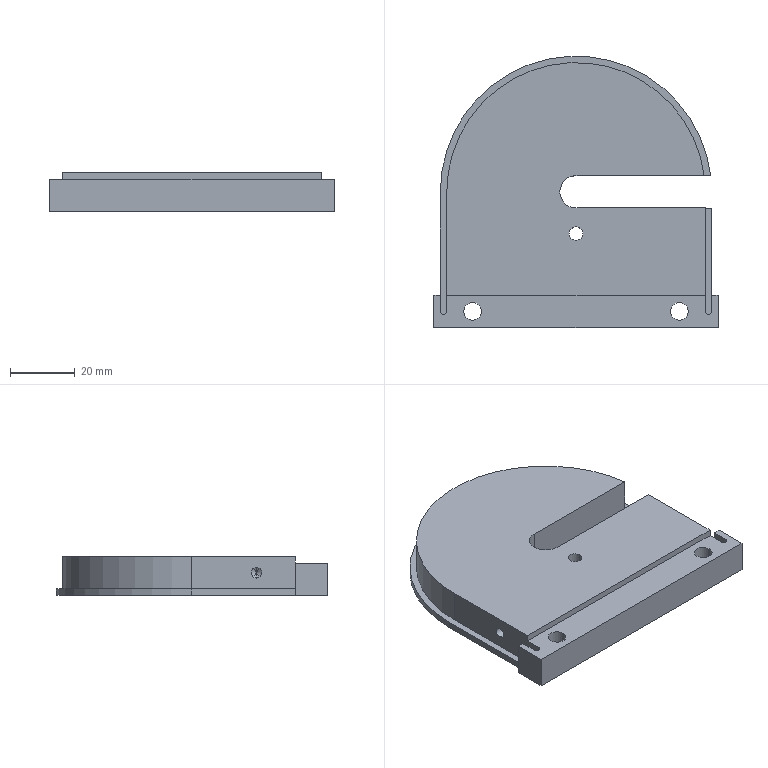Part | SolidWorks | features ICE 6, 3DProfileFeature 3, HoleWzd 3, Extrusion 1 | 1 solid | 45 faces | box 88 x 84 x 12 mm | volume 63664 mm3 | plane 21 | cylinder 20 | cone 4 | commonest cylinder face diameters 3.3 x4 5.5 x4 9 x4 2 x2 4.2 x2 10 x2
STEP:
#1=CARTESIAN_POINT('',(2.1,8.082,12.));
#2=VERTEX_POINT('',#1);
#3=CARTESIAN_POINT('',(-2.1,8.082,12.));
#4=VERTEX_POINT('',#3);
#5=CARTESIAN_POINT('',(0.,8.082,12.));
#6=DIRECTION('',(0.,0.,-1.));
#7=DIRECTION('',(-1.,0.,0.));
#8=AXIS2_PLACEMENT_3D('',#5,#6,#7);
#9=CIRCLE('',#8,2.1);
#10=EDGE_CURVE('',#2,#4,#9,.T.);
#11=ORIENTED_EDGE('',*,*,#10,.F.);
#12=CARTESIAN_POINT('',(2.1,8.082,0.));
#13=VERTEX_POINT('',#12);
#14=CARTESIAN_POINT('',(2.1,8.082,0.));
#15=DIRECTION('',(0.,0.,-1.));
#16=VECTOR('',#15,1000.);
#17=LINE('',#14,#16);
#18=EDGE_CURVE('',#2,#13,#17,.T.);
#19=ORIENTED_EDGE('',*,*,#18,.T.);
#20=CARTESIAN_POINT('',(-2.1,8.082,0.));
#21=VERTEX_POINT('',#20);
#22=CARTESIAN_POINT('',(0.,8.082,0.));
#23=DIRECTION('',(0.,0.,-1.));
#24=DIRECTION('',(-1.,0.,0.));
#25=AXIS2_PLACEMENT_3D('',#22,#23,#24);
#26=CIRCLE('',#25,2.1);
#27=EDGE_CURVE('',#13,#21,#26,.T.);
#28=ORIENTED_EDGE('',*,*,#27,.T.);
#29=CARTESIAN_POINT('',(-2.1,8.082,0.));
#30=DIRECTION('',(0.,0.,-1.));
#31=VECTOR('',#30,1000.);
#32=LINE('',#29,#31);
#33=EDGE_CURVE('',#4,#21,#32,.T.);
#34=ORIENTED_EDGE('',*,*,#33,.F.);
#35=EDGE_LOOP('',(#11,#19,#28,#34));
#36=FACE_OUTER_BOUND('',#35,.T.);
#37=CARTESIAN_POINT('',(0.,8.082,0.));
#38=DIRECTION('',(0.,0.,-1.));
#39=DIRECTION('',(-1.,0.,0.));
#40=AXIS2_PLACEMENT_3D('',#37,#38,#39);
#41=CYLINDRICAL_SURFACE('',#40,2.1);
#42=ADVANCED_FACE('',(#36),#41,.F.);
#43=CARTESIAN_POINT('',(30.,1.,8.665));
#44=VERTEX_POINT('',#43);
#45=CARTESIAN_POINT('',(30.,1.,5.365));
#46=VERTEX_POINT('',#45);
#47=CARTESIAN_POINT('',(30.,1.,7.015));
#48=DIRECTION('',(1.,0.,0.));
#49=DIRECTION('',(0.,0.,-1.));
#50=AXIS2_PLACEMENT_3D('',#47,#48,#49);
#51=CIRCLE('',#50,1.65);
#52=EDGE_CURVE('',#44,#46,#51,.T.);
#53=ORIENTED_EDGE('',*,*,#52,.F.);
#54=CARTESIAN_POINT('',(40.,1.,8.665));
#55=VERTEX_POINT('',#54);
#56=CARTESIAN_POINT('',(40.,1.,8.665));
#57=DIRECTION('',(1.,0.,0.));
#58=VECTOR('',#57,1000.);
#59=LINE('',#56,#58);
#60=EDGE_CURVE('',#44,#55,#59,.T.);
#61=ORIENTED_EDGE('',*,*,#60,.T.);
#62=CARTESIAN_POINT('',(40.,1.,5.365));
#63=VERTEX_POINT('',#62);
#64=CARTESIAN_POINT('',(40.,1.,7.015));
#65=DIRECTION('',(1.,0.,0.));
#66=DIRECTION('',(0.,0.,-1.));
#67=AXIS2_PLACEMENT_3D('',#64,#65,#66);
#68=CIRCLE('',#67,1.65);
#69=EDGE_CURVE('',#55,#63,#68,.T.);
#70=ORIENTED_EDGE('',*,*,#69,.T.);
#71=CARTESIAN_POINT('',(40.,1.,5.365));
#72=DIRECTION('',(1.,0.,0.));
#73=VECTOR('',#72,1000.);
#74=LINE('',#71,#73);
#75=EDGE_CURVE('',#46,#63,#74,.T.);
#76=ORIENTED_EDGE('',*,*,#75,.F.);
#77=EDGE_LOOP('',(#53,#61,#70,#76));
#78=FACE_OUTER_BOUND('',#77,.T.);
#79=CARTESIAN_POINT('',(40.,1.,7.015));
#80=DIRECTION('',(1.,0.,0.));
#81=DIRECTION('',(0.,0.,-1.));
#82=AXIS2_PLACEMENT_3D('',#79,#80,#81);
#83=CYLINDRICAL_SURFACE('',#82,1.65);
#84=ADVANCED_FACE('',(#78),#83,.F.);
#85=CARTESIAN_POINT('',(29.009,1.,7.015));
#86=VERTEX_POINT('',#85);
#87=CARTESIAN_POINT('',(30.,1.,5.365));
#88=DIRECTION('',(0.515,0.,-0.8572));
#89=VECTOR('',#88,1000.);
#90=LINE('',#87,#89);
#91=EDGE_CURVE('',#86,#46,#90,.T.);
#92=ORIENTED_EDGE('',*,*,#91,.F.);
#93=CARTESIAN_POINT('',(30.,1.,8.665));
#94=DIRECTION('',(0.515,0.,0.8572));
#95=VECTOR('',#94,1000.);
#96=LINE('',#93,#95);
#97=EDGE_CURVE('',#86,#44,#96,.T.);
#98=ORIENTED_EDGE('',*,*,#97,.T.);
#99=ORIENTED_EDGE('',*,*,#52,.T.);
#100=EDGE_LOOP('',(#92,#98,#99));
#101=FACE_OUTER_BOUND('',#100,.T.);
#102=CARTESIAN_POINT('',(30.,1.,7.015));
#103=DIRECTION('',(1.,0.,0.));
#104=DIRECTION('',(0.,0.,-1.));
#105=AXIS2_PLACEMENT_3D('',#102,#103,#104);
#106=CONICAL_SURFACE('',#105,1.65,1.03);
#107=ADVANCED_FACE('',(#101),#106,.F.);
#108=CARTESIAN_POINT('',(-30.,1.,5.35));
#109=VERTEX_POINT('',#108);
#110=CARTESIAN_POINT('',(-30.,1.,8.65));
#111=VERTEX_POINT('',#110);
#112=CARTESIAN_POINT('',(-30.,1.,7.));
#113=DIRECTION('',(-1.,0.,0.));
#114=DIRECTION('',(0.,0.,1.));
#115=AXIS2_PLACEMENT_3D('',#112,#113,#114);
#116=CIRCLE('',#115,1.65);
#117=EDGE_CURVE('',#109,#111,#116,.T.);
#118=ORIENTED_EDGE('',*,*,#117,.F.);
#119=CARTESIAN_POINT('',(-40.,1.,5.35));
#120=VERTEX_POINT('',#119);
#121=CARTESIAN_POINT('',(-40.,1.,5.35));
#122=DIRECTION('',(-1.,0.,0.));
#123=VECTOR('',#122,1000.);
#124=LINE('',#121,#123);
#125=EDGE_CURVE('',#109,#120,#124,.T.);
#126=ORIENTED_EDGE('',*,*,#125,.T.);
#127=CARTESIAN_POINT('',(-40.,1.,8.65));
#128=VERTEX_POINT('',#127);
#129=CARTESIAN_POINT('',(-40.,1.,7.));
#130=DIRECTION('',(-1.,0.,0.));
#131=DIRECTION('',(0.,0.,1.));
#132=AXIS2_PLACEMENT_3D('',#129,#130,#131);
#133=CIRCLE('',#132,1.65);
#134=EDGE_CURVE('',#120,#128,#133,.T.);
#135=ORIENTED_EDGE('',*,*,#134,.T.);
#136=CARTESIAN_POINT('',(-40.,1.,8.65));
#137=DIRECTION('',(-1.,0.,0.));
#138=VECTOR('',#137,1000.);
#139=LINE('',#136,#138);
#140=EDGE_CURVE('',#111,#128,#139,.T.);
#141=ORIENTED_EDGE('',*,*,#140,.F.);
#142=EDGE_LOOP('',(#118,#126,#135,#141));
#143=FACE_OUTER_BOUND('',#142,.T.);
#144=CARTESIAN_POINT('',(-40.,1.,7.));
#145=DIRECTION('',(-1.,0.,0.));
#146=DIRECTION('',(0.,0.,1.));
#147=AXIS2_PLACEMENT_3D('',#144,#145,#146);
#148=CYLINDRICAL_SURFACE('',#147,1.65);
#149=ADVANCED_FACE('',(#143),#148,.F.);
#150=CARTESIAN_POINT('',(-29.009,1.,7.));
#151=VERTEX_POINT('',#150);
#152=CARTESIAN_POINT('',(-30.,1.,8.65));
#153=DIRECTION('',(-0.515,0.,0.8572));
#154=VECTOR('',#153,1000.);
#155=LINE('',#152,#154);
#156=EDGE_CURVE('',#151,#111,#155,.T.);
#157=ORIENTED_EDGE('',*,*,#156,.F.);
#158=CARTESIAN_POINT('',(-30.,1.,5.35));
#159=DIRECTION('',(-0.515,0.,-0.8572));
#160=VECTOR('',#159,1000.);
#161=LINE('',#158,#160);
#162=EDGE_CURVE('',#151,#109,#161,.T.);
#163=ORIENTED_EDGE('',*,*,#162,.T.);
#164=ORIENTED_EDGE('',*,*,#117,.T.);
#165=EDGE_LOOP('',(#157,#163,#164));
#166=FACE_OUTER_BOUND('',#165,.T.);
#167=CARTESIAN_POINT('',(-30.,1.,7.));
#168=DIRECTION('',(-1.,0.,0.));
#169=DIRECTION('',(0.,0.,1.));
#170=AXIS2_PLACEMENT_3D('',#167,#168,#169);
#171=CONICAL_SURFACE('',#170,1.65,1.03);
#172=ADVANCED_FACE('',(#166),#171,.F.);
#173=CARTESIAN_POINT('',(-27.5,-16.,6.));
#174=VERTEX_POINT('',#173);
#175=CARTESIAN_POINT('',(-36.5,-16.,6.));
#176=VERTEX_POINT('',#175);
#177=CARTESIAN_POINT('',(-32.,-16.,6.));
#178=DIRECTION('',(0.,0.,-1.));
#179=DIRECTION('',(-1.,0.,0.));
#180=AXIS2_PLACEMENT_3D('',#177,#178,#179);
#181=CIRCLE('',#180,4.5);
#182=EDGE_CURVE('',#174,#176,#181,.T.);
#183=ORIENTED_EDGE('',*,*,#182,.F.);
#184=CARTESIAN_POINT('',(-27.5,-16.,0.));
#185=VERTEX_POINT('',#184);
#186=CARTESIAN_POINT('',(-27.5,-16.,6.));
#187=DIRECTION('',(0.,0.,-1.));
#188=VECTOR('',#187,1000.);
#189=LINE('',#186,#188);
#190=EDGE_CURVE('',#174,#185,#189,.T.);
#191=ORIENTED_EDGE('',*,*,#190,.T.);
#192=CARTESIAN_POINT('',(-36.5,-16.,0.));
#193=VERTEX_POINT('',#192);
#194=CARTESIAN_POINT('',(-32.,-16.,0.));
#195=DIRECTION('',(0.,0.,-1.));
#196=DIRECTION('',(-1.,0.,0.));
#197=AXIS2_PLACEMENT_3D('',#194,#195,#196);
#198=CIRCLE('',#197,4.5);
#199=EDGE_CURVE('',#185,#193,#198,.T.);
#200=ORIENTED_EDGE('',*,*,#199,.T.);
#201=CARTESIAN_POINT('',(-36.5,-16.,6.));
#202=DIRECTION('',(0.,0.,-1.));
#203=VECTOR('',#202,1000.);
#204=LINE('',#201,#203);
#205=EDGE_CURVE('',#176,#193,#204,.T.);
#206=ORIENTED_EDGE('',*,*,#205,.F.);
#207=EDGE_LOOP('',(#183,#191,#200,#206));
#208=FACE_OUTER_BOUND('',#207,.T.);
#209=CARTESIAN_POINT('',(-32.,-16.,6.));
#210=DIRECTION('',(0.,0.,-1.));
#211=DIRECTION('',(-1.,0.,0.));
#212=AXIS2_PLACEMENT_3D('',#209,#210,#211);
#213=CYLINDRICAL_SURFACE('',#212,4.5);
#214=ADVANCED_FACE('',(#208),#213,.F.);
#215=CARTESIAN_POINT('',(36.5,-16.,6.));
#216=VERTEX_POINT('',#215);
#217=CARTESIAN_POINT('',(27.5,-16.,6.));
#218=VERTEX_POINT('',#217);
#219=CARTESIAN_POINT('',(32.,-16.,6.));
#220=DIRECTION('',(0.,0.,-1.));
#221=DIRECTION('',(-1.,0.,0.));
#222=AXIS2_PLACEMENT_3D('',#219,#220,#221);
#223=CIRCLE('',#222,4.5);
#224=EDGE_CURVE('',#216,#218,#223,.T.);
#225=ORIENTED_EDGE('',*,*,#224,.F.);
#226=CARTESIAN_POINT('',(36.5,-16.,0.));
#227=VERTEX_POINT('',#226);
#228=CARTESIAN_POINT('',(36.5,-16.,6.));
#229=DIRECTION('',(0.,0.,-1.));
#230=VECTOR('',#229,1000.);
#231=LINE('',#228,#230);
#232=EDGE_CURVE('',#216,#227,#231,.T.);
#233=ORIENTED_EDGE('',*,*,#232,.T.);
#234=CARTESIAN_POINT('',(27.5,-16.,0.));
#235=VERTEX_POINT('',#234);
#236=CARTESIAN_POINT('',(32.,-16.,0.));
#237=DIRECTION('',(0.,0.,-1.));
#238=DIRECTION('',(-1.,0.,0.));
#239=AXIS2_PLACEMENT_3D('',#236,#237,#238);
#240=CIRCLE('',#239,4.5);
#241=EDGE_CURVE('',#227,#235,#240,.T.);
#242=ORIENTED_EDGE('',*,*,#241,.T.);
#243=CARTESIAN_POINT('',(27.5,-16.,6.));
#244=DIRECTION('',(0.,0.,-1.));
#245=VECTOR('',#244,1000.);
#246=LINE('',#243,#245);
#247=EDGE_CURVE('',#218,#235,#246,.T.);
#248=ORIENTED_EDGE('',*,*,#247,.F.);
#249=EDGE_LOOP('',(#225,#233,#242,#248));
#250=FACE_OUTER_BOUND('',#249,.T.);
#251=CARTESIAN_POINT('',(32.,-16.,6.));
#252=DIRECTION('',(0.,0.,-1.));
#253=DIRECTION('',(-1.,0.,0.));
#254=AXIS2_PLACEMENT_3D('',#251,#252,#253);
#255=CYLINDRICAL_SURFACE('',#254,4.5);
#256=ADVANCED_FACE('',(#250),#255,.F.);
#257=CARTESIAN_POINT('',(-5.,21.,12.));
#258=VERTEX_POINT('',#257);
#259=CARTESIAN_POINT('',(0.,26.,12.));
#260=VERTEX_POINT('',#259);
#261=CARTESIAN_POINT('',(0.,21.,12.));
#262=DIRECTION('',(0.,0.,-1.));
#263=DIRECTION('',(-1.,0.,0.));
#264=AXIS2_PLACEMENT_3D('',#261,#262,#263);
#265=CIRCLE('',#264,5.);
#266=EDGE_CURVE('',#258,#260,#265,.T.);
#267=ORIENTED_EDGE('',*,*,#266,.F.);
#268=CARTESIAN_POINT('',(-5.,21.,0.));
#269=VERTEX_POINT('',#268);
#270=CARTESIAN_POINT('',(-5.,21.,12.));
#271=DIRECTION('',(0.,0.,-1.));
#272=VECTOR('',#271,1000.);
#273=LINE('',#270,#272);
#274=EDGE_CURVE('',#258,#269,#273,.T.);
#275=ORIENTED_EDGE('',*,*,#274,.T.);
#276=CARTESIAN_POINT('',(0.,26.,0.));
#277=VERTEX_POINT('',#276);
#278=CARTESIAN_POINT('',(0.,21.,0.));
#279=DIRECTION('',(0.,0.,-1.));
#280=DIRECTION('',(-1.,0.,0.));
#281=AXIS2_PLACEMENT_3D('',#278,#279,#280);
#282=CIRCLE('',#281,5.);
#283=EDGE_CURVE('',#269,#277,#282,.T.);
#284=ORIENTED_EDGE('',*,*,#283,.T.);
#285=CARTESIAN_POINT('',(0.,26.,12.));
#286=DIRECTION('',(0.,0.,-1.));
#287=VECTOR('',#286,1000.);
#288=LINE('',#285,#287);
#289=EDGE_CURVE('',#260,#277,#288,.T.);
#290=ORIENTED_EDGE('',*,*,#289,.F.);
#291=EDGE_LOOP('',(#267,#275,#284,#290));
#292=FACE_OUTER_BOUND('',#291,.T.);
#293=CARTESIAN_POINT('',(0.,21.,12.));
#294=DIRECTION('',(0.,0.,-1.));
#295=DIRECTION('',(-1.,0.,0.));
#296=AXIS2_PLACEMENT_3D('',#293,#294,#295);
#297=CYLINDRICAL_SURFACE('',#296,5.);
#298=ADVANCED_FACE('',(#292),#297,.F.);
#299=CARTESIAN_POINT('',(34.75,-16.,10.));
#300=VERTEX_POINT('',#299);
#301=CARTESIAN_POINT('',(29.25,-16.,10.));
#302=VERTEX_POINT('',#301);
#303=CARTESIAN_POINT('',(32.,-16.,10.));
#304=DIRECTION('',(0.,0.,-1.));
#305=DIRECTION('',(-1.,0.,0.));
#306=AXIS2_PLACEMENT_3D('',#303,#304,#305);
#307=CIRCLE('',#306,2.75);
#308=EDGE_CURVE('',#300,#302,#307,.T.);
#309=ORIENTED_EDGE('',*,*,#308,.F.);
#310=CARTESIAN_POINT('',(34.75,-16.,6.));
#311=VERTEX_POINT('',#310);
#312=CARTESIAN_POINT('',(34.75,-16.,12.));
#313=DIRECTION('',(0.,0.,-1.));
#314=VECTOR('',#313,1000.);
#315=LINE('',#312,#314);
#316=EDGE_CURVE('',#300,#311,#315,.T.);
#317=ORIENTED_EDGE('',*,*,#316,.T.);
#318=CARTESIAN_POINT('',(29.25,-16.,6.));
#319=VERTEX_POINT('',#318);
#320=CARTESIAN_POINT('',(32.,-16.,6.));
#321=DIRECTION('',(0.,0.,1.));
#322=DIRECTION('',(-1.,0.,0.));
#323=AXIS2_PLACEMENT_3D('',#320,#321,#322);
#324=CIRCLE('',#323,2.75);
#325=EDGE_CURVE('',#319,#311,#324,.T.);
#326=ORIENTED_EDGE('',*,*,#325,.F.);
#327=CARTESIAN_POINT('',(29.25,-16.,12.));
#328=DIRECTION('',(0.,0.,-1.));
#329=VECTOR('',#328,1000.);
#330=LINE('',#327,#329);
#331=EDGE_CURVE('',#302,#319,#330,.T.);
#332=ORIENTED_EDGE('',*,*,#331,.F.);
#333=EDGE_LOOP('',(#309,#317,#326,#332));
#334=FACE_OUTER_BOUND('',#333,.T.);
#335=CARTESIAN_POINT('',(32.,-16.,12.));
#336=DIRECTION('',(0.,0.,-1.));
#337=DIRECTION('',(-1.,0.,0.));
#338=AXIS2_PLACEMENT_3D('',#335,#336,#337);
#339=CYLINDRICAL_SURFACE('',#338,2.75);
#340=ADVANCED_FACE('',(#334),#339,.F.);
#341=CARTESIAN_POINT('',(-29.25,-16.,10.));
#342=VERTEX_POINT('',#341);
#343=CARTESIAN_POINT('',(-34.75,-16.,10.));
#344=VERTEX_POINT('',#343);
#345=CARTESIAN_POINT('',(-32.,-16.,10.));
#346=DIRECTION('',(0.,0.,-1.));
#347=DIRECTION('',(-1.,0.,0.));
#348=AXIS2_PLACEMENT_3D('',#345,#346,#347);
#349=CIRCLE('',#348,2.75);
#350=EDGE_CURVE('',#342,#344,#349,.T.);
#351=ORIENTED_EDGE('',*,*,#350,.F.);
#352=CARTESIAN_POINT('',(-29.25,-16.,6.));
#353=VERTEX_POINT('',#352);
#354=CARTESIAN_POINT('',(-29.25,-16.,12.));
#355=DIRECTION('',(0.,0.,-1.));
#356=VECTOR('',#355,1000.);
#357=LINE('',#354,#356);
#358=EDGE_CURVE('',#342,#353,#357,.T.);
#359=ORIENTED_EDGE('',*,*,#358,.T.);
#360=CARTESIAN_POINT('',(-34.75,-16.,6.));
#361=VERTEX_POINT('',#360);
#362=CARTESIAN_POINT('',(-32.,-16.,6.));
#363=DIRECTION('',(0.,0.,1.));
#364=DIRECTION('',(-1.,0.,0.));
#365=AXIS2_PLACEMENT_3D('',#362,#363,#364);
#366=CIRCLE('',#365,2.75);
#367=EDGE_CURVE('',#361,#353,#366,.T.);
#368=ORIENTED_EDGE('',*,*,#367,.F.);
#369=CARTESIAN_POINT('',(-34.75,-16.,12.));
#370=DIRECTION('',(0.,0.,-1.));
#371=VECTOR('',#370,1000.);
#372=LINE('',#369,#371);
#373=EDGE_CURVE('',#344,#361,#372,.T.);
#374=ORIENTED_EDGE('',*,*,#373,.F.);
#375=EDGE_LOOP('',(#351,#359,#368,#374));
#376=FACE_OUTER_BOUND('',#375,.T.);
#377=CARTESIAN_POINT('',(-32.,-16.,12.));
#378=DIRECTION('',(0.,0.,-1.));
#379=DIRECTION('',(-1.,0.,0.));
#380=AXIS2_PLACEMENT_3D('',#377,#378,#379);
#381=CYLINDRICAL_SURFACE('',#380,2.75);
#382=ADVANCED_FACE('',(#376),#381,.F.);
#383=ORIENTED_EDGE('',*,*,#358,.F.);
#384=CARTESIAN_POINT('',(-32.,-16.,10.));
#385=DIRECTION('',(0.,0.,-1.));
#386=DIRECTION('',(-1.,0.,0.));
#387=AXIS2_PLACEMENT_3D('',#384,#385,#386);
#388=CIRCLE('',#387,2.75);
#389=EDGE_CURVE('',#344,#342,#388,.T.);
#390=ORIENTED_EDGE('',*,*,#389,.F.);
#391=ORIENTED_EDGE('',*,*,#373,.T.);
#392=CARTESIAN_POINT('',(-32.,-16.,6.));
#393=DIRECTION('',(0.,0.,1.));
#394=DIRECTION('',(-1.,0.,0.));
#395=AXIS2_PLACEMENT_3D('',#392,#393,#394);
#396=CIRCLE('',#395,2.75);
#397=EDGE_CURVE('',#353,#361,#396,.T.);
#398=ORIENTED_EDGE('',*,*,#397,.F.);
#399=EDGE_LOOP('',(#383,#390,#391,#398));
#400=FACE_OUTER_BOUND('',#399,.T.);
#401=CARTESIAN_POINT('',(-32.,-16.,12.));
#402=DIRECTION('',(0.,0.,-1.));
#403=DIRECTION('',(-1.,0.,0.));
#404=AXIS2_PLACEMENT_3D('',#401,#402,#403);
#405=CYLINDRICAL_SURFACE('',#404,2.75);
#406=ADVANCED_FACE('',(#400),#405,.F.);
#407=ORIENTED_EDGE('',*,*,#316,.F.);
#408=CARTESIAN_POINT('',(32.,-16.,10.));
#409=DIRECTION('',(0.,0.,-1.));
#410=DIRECTION('',(-1.,0.,0.));
#411=AXIS2_PLACEMENT_3D('',#408,#409,#410);
#412=CIRCLE('',#411,2.75);
#413=EDGE_CURVE('',#302,#300,#412,.T.);
#414=ORIENTED_EDGE('',*,*,#413,.F.);
#415=ORIENTED_EDGE('',*,*,#331,.T.);
#416=CARTESIAN_POINT('',(32.,-16.,6.));
#417=DIRECTION('',(0.,0.,1.));
#418=DIRECTION('',(-1.,0.,0.));
#419=AXIS2_PLACEMENT_3D('',#416,#417,#418);
#420=CIRCLE('',#419,2.75);
#421=EDGE_CURVE('',#311,#319,#420,.T.);
#422=ORIENTED_EDGE('',*,*,#421,.F.);
#423=EDGE_LOOP('',(#407,#414,#415,#422));
#424=FACE_OUTER_BOUND('',#423,.T.);
#425=CARTESIAN_POINT('',(32.,-16.,12.));
#426=DIRECTION('',(0.,0.,-1.));
#427=DIRECTION('',(-1.,0.,0.));
#428=AXIS2_PLACEMENT_3D('',#425,#426,#427);
#429=CYLINDRICAL_SURFACE('',#428,2.75);
#430=ADVANCED_FACE('',(#424),#429,.F.);
#431=CARTESIAN_POINT('',(40.,16.,2.));
#432=VERTEX_POINT('',#431);
#433=CARTESIAN_POINT('',(42.,16.,2.));
#434=VERTEX_POINT('',#433);
#435=CARTESIAN_POINT('',(0.,16.,2.));
#436=DIRECTION('',(1.,0.,0.));
#437=VECTOR('',#436,1000.);
#438=LINE('',#435,#437);
#439=EDGE_CURVE('',#432,#434,#438,.T.);
#440=ORIENTED_EDGE('',*,*,#439,.F.);
#441=CARTESIAN_POINT('',(40.,-16.,2.));
#442=VERTEX_POINT('',#441);
#443=CARTESIAN_POINT('',(40.,-11.,2.));
#444=DIRECTION('',(0.,-1.,0.));
#445=VECTOR('',#444,1000.);
#446=LINE('',#443,#445);
#447=EDGE_CURVE('',#432,#442,#446,.T.);
#448=ORIENTED_EDGE('',*,*,#447,.T.);
#449=CARTESIAN_POINT('',(42.,-16.,2.));
#450=VERTEX_POINT('',#449);
#451=CARTESIAN_POINT('',(41.,-16.,2.));
#452=DIRECTION('',(0.,0.,1.));
#453=DIRECTION('',(1.,0.,0.));
#454=AXIS2_PLACEMENT_3D('',#451,#452,#453);
#455=CIRCLE('',#454,1.);
#456=EDGE_CURVE('',#442,#450,#455,.T.);
#457=ORIENTED_EDGE('',*,*,#456,.T.);
#458=CARTESIAN_POINT('',(42.,-11.,2.));
#459=VERTEX_POINT('',#458);
#460=CARTESIAN_POINT('',(42.,-11.,2.));
#461=DIRECTION('',(0.,1.,0.));
#462=VECTOR('',#461,1000.);
#463=LINE('',#460,#462);
#464=EDGE_CURVE('',#450,#459,#463,.T.);
#465=ORIENTED_EDGE('',*,*,#464,.T.);
#466=CARTESIAN_POINT('',(42.,21.,2.));
#467=DIRECTION('',(0.,1.,0.));
#468=VECTOR('',#467,1000.);
#469=LINE('',#466,#468);
#470=EDGE_CURVE('',#459,#434,#469,.T.);
#471=ORIENTED_EDGE('',*,*,#470,.T.);
#472=EDGE_LOOP('',(#440,#448,#457,#465,#471));
#473=FACE_OUTER_BOUND('',#472,.T.);
#474=CARTESIAN_POINT('',(0.,21.,2.));
#475=DIRECTION('',(0.,0.,1.));
#476=DIRECTION('',(1.,0.,0.));
#477=AXIS2_PLACEMENT_3D('',#474,#475,#476);
#478=PLANE('',#477);
#479=ADVANCED_FACE('',(#473),#478,.T.);
#480=CARTESIAN_POINT('',(42.,-11.,0.));
#481=VERTEX_POINT('',#480);
#482=CARTESIAN_POINT('',(42.,16.,0.));
#483=VERTEX_POINT('',#482);
#484=CARTESIAN_POINT('',(42.,21.,0.));
#485=DIRECTION('',(0.,1.,0.));
#486=VECTOR('',#485,1000.);
#487=LINE('',#484,#486);
#488=EDGE_CURVE('',#481,#483,#487,.T.);
#489=ORIENTED_EDGE('',*,*,#488,.T.);
#490=CARTESIAN_POINT('',(42.,16.,12.));
#491=DIRECTION('',(0.,0.,1.));
#492=VECTOR('',#491,1000.);
#493=LINE('',#490,#492);
#494=EDGE_CURVE('',#483,#434,#493,.T.);
#495=ORIENTED_EDGE('',*,*,#494,.T.);
#496=ORIENTED_EDGE('',*,*,#470,.F.);
#497=CARTESIAN_POINT('',(42.,-11.,12.));
#498=DIRECTION('',(0.,0.,-1.));
#499=VECTOR('',#498,1000.);
#500=LINE('',#497,#499);
#501=EDGE_CURVE('',#459,#481,#500,.T.);
#502=ORIENTED_EDGE('',*,*,#501,.T.);
#503=EDGE_LOOP('',(#489,#495,#496,#502));
#504=FACE_OUTER_BOUND('',#503,.T.);
#505=CARTESIAN_POINT('',(42.,21.,12.));
#506=DIRECTION('',(-1.,0.,0.));
#507=DIRECTION('',(0.,0.,1.));
#508=AXIS2_PLACEMENT_3D('',#505,#506,#507);
#509=PLANE('',#508);
#510=ADVANCED_FACE('',(#504),#509,.F.);
#511=CARTESIAN_POINT('',(41.701,26.,2.));
#512=VERTEX_POINT('',#511);
#513=CARTESIAN_POINT('',(-42.,21.,2.));
#514=VERTEX_POINT('',#513);
#515=CARTESIAN_POINT('',(0.,21.,2.));
#516=DIRECTION('',(0.,0.,1.));
#517=DIRECTION('',(1.,0.,0.));
#518=AXIS2_PLACEMENT_3D('',#515,#516,#517);
#519=CIRCLE('',#518,42.);
#520=EDGE_CURVE('',#512,#514,#519,.T.);
#521=ORIENTED_EDGE('',*,*,#520,.F.);
#522=CARTESIAN_POINT('',(41.701,26.,0.));
#523=VERTEX_POINT('',#522);
#524=CARTESIAN_POINT('',(41.701,26.,12.));
#525=DIRECTION('',(0.,0.,-1.));
#526=VECTOR('',#525,1000.);
#527=LINE('',#524,#526);
#528=EDGE_CURVE('',#512,#523,#527,.T.);
#529=ORIENTED_EDGE('',*,*,#528,.T.);
#530=CARTESIAN_POINT('',(-42.,21.,0.));
#531=VERTEX_POINT('',#530);
#532=CARTESIAN_POINT('',(0.,21.,0.));
#533=DIRECTION('',(0.,0.,1.));
#534=DIRECTION('',(1.,0.,0.));
#535=AXIS2_PLACEMENT_3D('',#532,#533,#534);
#536=CIRCLE('',#535,42.);
#537=EDGE_CURVE('',#523,#531,#536,.T.);
#538=ORIENTED_EDGE('',*,*,#537,.T.);
#539=CARTESIAN_POINT('',(-42.,21.,12.));
#540=DIRECTION('',(0.,0.,-1.));
#541=VECTOR('',#540,1000.);
#542=LINE('',#539,#541);
#543=EDGE_CURVE('',#514,#531,#542,.T.);
#544=ORIENTED_EDGE('',*,*,#543,.F.);
#545=EDGE_LOOP('',(#521,#529,#538,#544));
#546=FACE_OUTER_BOUND('',#545,.T.);
#547=CARTESIAN_POINT('',(0.,21.,12.));
#548=DIRECTION('',(0.,0.,-1.));
#549=DIRECTION('',(-1.,0.,0.));
#550=AXIS2_PLACEMENT_3D('',#547,#548,#549);
#551=CYLINDRICAL_SURFACE('',#550,42.);
#552=ADVANCED_FACE('',(#546),#551,.T.);
#553=CARTESIAN_POINT('',(-42.,-11.,2.));
#554=VERTEX_POINT('',#553);
#555=CARTESIAN_POINT('',(-42.,21.,2.));
#556=DIRECTION('',(0.,-1.,0.));
#557=VECTOR('',#556,1000.);
#558=LINE('',#555,#557);
#559=EDGE_CURVE('',#514,#554,#558,.T.);
#560=ORIENTED_EDGE('',*,*,#559,.F.);
#561=ORIENTED_EDGE('',*,*,#543,.T.);
#562=CARTESIAN_POINT('',(-42.,-11.,0.));
#563=VERTEX_POINT('',#562);
#564=CARTESIAN_POINT('',(-42.,21.,0.));
#565=DIRECTION('',(0.,-1.,0.));
#566=VECTOR('',#565,1000.);
#567=LINE('',#564,#566);
#568=EDGE_CURVE('',#531,#563,#567,.T.);
#569=ORIENTED_EDGE('',*,*,#568,.T.);
#570=CARTESIAN_POINT('',(-42.,-11.,12.));
#571=DIRECTION('',(0.,0.,-1.));
#572=VECTOR('',#571,1000.);
#573=LINE('',#570,#572);
#574=EDGE_CURVE('',#554,#563,#573,.T.);
#575=ORIENTED_EDGE('',*,*,#574,.F.);
#576=EDGE_LOOP('',(#560,#561,#569,#575));
#577=FACE_OUTER_BOUND('',#576,.T.);
#578=CARTESIAN_POINT('',(-42.,21.,12.));
#579=DIRECTION('',(1.,0.,0.));
#580=DIRECTION('',(0.,0.,-1.));
#581=AXIS2_PLACEMENT_3D('',#578,#579,#580);
#582=PLANE('',#581);
#583=ADVANCED_FACE('',(#577),#582,.F.);
#584=CARTESIAN_POINT('',(44.,-11.,10.));
#585=VERTEX_POINT('',#584);
#586=CARTESIAN_POINT('',(44.,-11.,0.));
#587=VERTEX_POINT('',#586);
#588=CARTESIAN_POINT('',(44.,-11.,12.));
#589=DIRECTION('',(0.,0.,-1.));
#590=VECTOR('',#589,1000.);
#591=LINE('',#588,#590);
#592=EDGE_CURVE('',#585,#587,#591,.T.);
#593=ORIENTED_EDGE('',*,*,#592,.F.);
#594=CARTESIAN_POINT('',(44.,-21.,10.));
#595=VERTEX_POINT('',#594);
#596=CARTESIAN_POINT('',(44.,-21.,10.));
#597=DIRECTION('',(0.,1.,0.));
#598=VECTOR('',#597,1000.);
#599=LINE('',#596,#598);
#600=EDGE_CURVE('',#595,#585,#599,.T.);
#601=ORIENTED_EDGE('',*,*,#600,.F.);
#602=CARTESIAN_POINT('',(44.,-21.,0.));
#603=VERTEX_POINT('',#602);
#604=CARTESIAN_POINT('',(44.,-21.,12.));
#605=DIRECTION('',(0.,0.,-1.));
#606=VECTOR('',#605,1000.);
#607=LINE('',#604,#606);
#608=EDGE_CURVE('',#595,#603,#607,.T.);
#609=ORIENTED_EDGE('',*,*,#608,.T.);
#610=CARTESIAN_POINT('',(44.,-11.,0.));
#611=DIRECTION('',(0.,1.,0.));
#612=VECTOR('',#611,1000.);
#613=LINE('',#610,#612);
#614=EDGE_CURVE('',#603,#587,#613,.T.);
#615=ORIENTED_EDGE('',*,*,#614,.T.);
#616=EDGE_LOOP('',(#593,#601,#609,#615));
#617=FACE_OUTER_BOUND('',#616,.T.);
#618=CARTESIAN_POINT('',(44.,-11.,12.));
#619=DIRECTION('',(-1.,0.,0.));
#620=DIRECTION('',(0.,0.,1.));
#621=AXIS2_PLACEMENT_3D('',#618,#619,#620);
#622=PLANE('',#621);
#623=ADVANCED_FACE('',(#617),#622,.F.);
#624=ORIENTED_EDGE('',*,*,#501,.F.);
#625=CARTESIAN_POINT('',(42.,-11.,10.));
#626=VERTEX_POINT('',#625);
#627=CARTESIAN_POINT('',(42.,-11.,2.));
#628=DIRECTION('',(0.,0.,1.));
#629=VECTOR('',#628,1000.);
#630=LINE('',#627,#629);
#631=EDGE_CURVE('',#459,#626,#630,.T.);
#632=ORIENTED_EDGE('',*,*,#631,.T.);
#633=CARTESIAN_POINT('',(-44.,-11.,10.));
#634=DIRECTION('',(1.,0.,0.));
#635=VECTOR('',#634,1000.);
#636=LINE('',#633,#635);
#637=EDGE_CURVE('',#626,#585,#636,.T.);
#638=ORIENTED_EDGE('',*,*,#637,.T.);
#639=ORIENTED_EDGE('',*,*,#592,.T.);
#640=CARTESIAN_POINT('',(44.,-11.,0.));
#641=DIRECTION('',(-1.,0.,0.));
#642=VECTOR('',#641,1000.);
#643=LINE('',#640,#642);
#644=EDGE_CURVE('',#587,#481,#643,.T.);
#645=ORIENTED_EDGE('',*,*,#644,.T.);
#646=EDGE_LOOP('',(#624,#632,#638,#639,#645));
#647=FACE_OUTER_BOUND('',#646,.T.);
#648=CARTESIAN_POINT('',(44.,-11.,12.));
#649=DIRECTION('',(0.,-1.,0.));
#650=DIRECTION('',(1.,0.,0.));
#651=AXIS2_PLACEMENT_3D('',#648,#649,#650);
#652=PLANE('',#651);
#653=ADVANCED_FACE('',(#647),#652,.F.);
#654=CARTESIAN_POINT('',(-44.,-11.,10.));
#655=VERTEX_POINT('',#654);
#656=CARTESIAN_POINT('',(-42.,-11.,10.));
#657=VERTEX_POINT('',#656);
#658=CARTESIAN_POINT('',(-44.,-11.,10.));
#659=DIRECTION('',(1.,0.,0.));
#660=VECTOR('',#659,1000.);
#661=LINE('',#658,#660);
#662=EDGE_CURVE('',#655,#657,#661,.T.);
#663=ORIENTED_EDGE('',*,*,#662,.T.);
#664=CARTESIAN_POINT('',(-42.,-11.,2.));
#665=DIRECTION('',(0.,0.,1.));
#666=VECTOR('',#665,1000.);
#667=LINE('',#664,#666);
#668=EDGE_CURVE('',#554,#657,#667,.T.);
#669=ORIENTED_EDGE('',*,*,#668,.F.);
#670=ORIENTED_EDGE('',*,*,#574,.T.);
#671=CARTESIAN_POINT('',(-44.,-11.,0.));
#672=VERTEX_POINT('',#671);
#673=CARTESIAN_POINT('',(-42.,-11.,0.));
#674=DIRECTION('',(-1.,0.,0.));
#675=VECTOR('',#674,1000.);
#676=LINE('',#673,#675);
#677=EDGE_CURVE('',#563,#672,#676,.T.);
#678=ORIENTED_EDGE('',*,*,#677,.T.);
#679=CARTESIAN_POINT('',(-44.,-11.,12.));
#680=DIRECTION('',(0.,0.,-1.));
#681=VECTOR('',#680,1000.);
#682=LINE('',#679,#681);
#683=EDGE_CURVE('',#655,#672,#682,.T.);
#684=ORIENTED_EDGE('',*,*,#683,.F.);
#685=EDGE_LOOP('',(#663,#669,#670,#678,#684));
#686=FACE_OUTER_BOUND('',#685,.T.);
#687=CARTESIAN_POINT('',(-42.,-11.,12.));
#688=DIRECTION('',(0.,-1.,0.));
#689=DIRECTION('',(1.,0.,0.));
#690=AXIS2_PLACEMENT_3D('',#687,#688,#689);
#691=PLANE('',#690);
#692=ADVANCED_FACE('',(#686),#691,.F.);
#693=CARTESIAN_POINT('',(-44.,-21.,10.));
#694=VERTEX_POINT('',#693);
#695=CARTESIAN_POINT('',(-44.,-21.,0.));
#696=VERTEX_POINT('',#695);
#697=CARTESIAN_POINT('',(-44.,-21.,12.));
#698=DIRECTION('',(0.,0.,-1.));
#699=VECTOR('',#698,1000.);
#700=LINE('',#697,#699);
#701=EDGE_CURVE('',#694,#696,#700,.T.);
#702=ORIENTED_EDGE('',*,*,#701,.F.);
#703=CARTESIAN_POINT('',(-44.,-21.,10.));
#704=DIRECTION('',(0.,1.,0.));
#705=VECTOR('',#704,1000.);
#706=LINE('',#703,#705);
#707=EDGE_CURVE('',#694,#655,#706,.T.);
#708=ORIENTED_EDGE('',*,*,#707,.T.);
#709=ORIENTED_EDGE('',*,*,#683,.T.);
#710=CARTESIAN_POINT('',(-44.,-11.,0.));
#711=DIRECTION('',(0.,-1.,0.));
#712=VECTOR('',#711,1000.);
#713=LINE('',#710,#712);
#714=EDGE_CURVE('',#672,#696,#713,.T.);
#715=ORIENTED_EDGE('',*,*,#714,.T.);
#716=EDGE_LOOP('',(#702,#708,#709,#715));
#717=FACE_OUTER_BOUND('',#716,.T.);
#718=CARTESIAN_POINT('',(-44.,-11.,12.));
#719=DIRECTION('',(1.,0.,0.));
#720=DIRECTION('',(0.,0.,-1.));
#721=AXIS2_PLACEMENT_3D('',#718,#719,#720);
#722=PLANE('',#721);
#723=ADVANCED_FACE('',(#717),#722,.F.);
#724=ORIENTED_EDGE('',*,*,#608,.F.);
#725=CARTESIAN_POINT('',(-44.,-21.,10.));
#726=DIRECTION('',(1.,0.,0.));
#727=VECTOR('',#726,1000.);
#728=LINE('',#725,#727);
#729=EDGE_CURVE('',#694,#595,#728,.T.);
#730=ORIENTED_EDGE('',*,*,#729,.F.);
#731=ORIENTED_EDGE('',*,*,#701,.T.);
#732=CARTESIAN_POINT('',(-44.,-21.,0.));
#733=DIRECTION('',(1.,0.,0.));
#734=VECTOR('',#733,1000.);
#735=LINE('',#732,#734);
#736=EDGE_CURVE('',#696,#603,#735,.T.);
#737=ORIENTED_EDGE('',*,*,#736,.T.);
#738=EDGE_LOOP('',(#724,#730,#731,#737));
#739=FACE_OUTER_BOUND('',#738,.T.);
#740=CARTESIAN_POINT('',(-44.,-21.,12.));
#741=DIRECTION('',(0.,1.,0.));
#742=DIRECTION('',(0.,0.,1.));
#743=AXIS2_PLACEMENT_3D('',#740,#741,#742);
#744=PLANE('',#743);
#745=ADVANCED_FACE('',(#739),#744,.F.);
#746=CARTESIAN_POINT('',(0.,8.082,12.));
#747=DIRECTION('',(0.,0.,-1.));
#748=DIRECTION('',(-1.,0.,0.));
#749=AXIS2_PLACEMENT_3D('',#746,#747,#748);
#750=CIRCLE('',#749,2.1);
#751=EDGE_CURVE('',#4,#2,#750,.T.);
#752=ORIENTED_EDGE('',*,*,#751,.T.);
#753=ORIENTED_EDGE('',*,*,#10,.T.);
#754=EDGE_LOOP('',(#752,#753));
#755=FACE_BOUND('',#754,.T.);
#756=CARTESIAN_POINT('',(40.,16.,12.));
#757=VERTEX_POINT('',#756);
#758=CARTESIAN_POINT('',(0.,16.,12.));
#759=VERTEX_POINT('',#758);
#760=CARTESIAN_POINT('',(46.264,16.,12.));
#761=DIRECTION('',(-1.,0.,0.));
#762=VECTOR('',#761,1000.);
#763=LINE('',#760,#762);
#764=EDGE_CURVE('',#757,#759,#763,.T.);
#765=ORIENTED_EDGE('',*,*,#764,.T.);
#766=CARTESIAN_POINT('',(0.,21.,12.));
#767=DIRECTION('',(0.,0.,-1.));
#768=DIRECTION('',(-1.,0.,0.));
#769=AXIS2_PLACEMENT_3D('',#766,#767,#768);
#770=CIRCLE('',#769,5.);
#771=EDGE_CURVE('',#759,#258,#770,.T.);
#772=ORIENTED_EDGE('',*,*,#771,.T.);
#773=ORIENTED_EDGE('',*,*,#266,.T.);
#774=CARTESIAN_POINT('',(39.686,26.,12.));
#775=VERTEX_POINT('',#774);
#776=CARTESIAN_POINT('',(0.,26.,12.));
#777=DIRECTION('',(1.,0.,0.));
#778=VECTOR('',#777,1000.);
#779=LINE('',#776,#778);
#780=EDGE_CURVE('',#260,#775,#779,.T.);
#781=ORIENTED_EDGE('',*,*,#780,.T.);
#782=CARTESIAN_POINT('',(-40.,21.,12.));
#783=VERTEX_POINT('',#782);
#784=CARTESIAN_POINT('',(0.,21.,12.));
#785=DIRECTION('',(0.,0.,-1.));
#786=DIRECTION('',(1.,0.,0.));
#787=AXIS2_PLACEMENT_3D('',#784,#785,#786);
#788=CIRCLE('',#787,40.);
#789=EDGE_CURVE('',#783,#775,#788,.T.);
#790=ORIENTED_EDGE('',*,*,#789,.F.);
#791=CARTESIAN_POINT('',(-40.,-11.,12.));
#792=VERTEX_POINT('',#791);
#793=CARTESIAN_POINT('',(-40.,21.,12.));
#794=DIRECTION('',(0.,1.,0.));
#795=VECTOR('',#794,1000.);
#796=LINE('',#793,#795);
#797=EDGE_CURVE('',#792,#783,#796,.T.);
#798=ORIENTED_EDGE('',*,*,#797,.F.);
#799=CARTESIAN_POINT('',(40.,-11.,12.));
#800=VERTEX_POINT('',#799);
#801=CARTESIAN_POINT('',(-44.,-11.,12.));
#802=DIRECTION('',(1.,0.,0.));
#803=VECTOR('',#802,1000.);
#804=LINE('',#801,#803);
#805=EDGE_CURVE('',#792,#800,#804,.T.);
#806=ORIENTED_EDGE('',*,*,#805,.T.);
#807=CARTESIAN_POINT('',(40.,-11.,12.));
#808=DIRECTION('',(0.,-1.,0.));
#809=VECTOR('',#808,1000.);
#810=LINE('',#807,#809);
#811=EDGE_CURVE('',#757,#800,#810,.T.);
#812=ORIENTED_EDGE('',*,*,#811,.F.);
#813=EDGE_LOOP('',(#765,#772,#773,#781,#790,#798,#806,#812));
#814=FACE_OUTER_BOUND('',#813,.T.);
#815=CARTESIAN_POINT('',(0.,21.,12.));
#816=DIRECTION('',(0.,0.,1.));
#817=DIRECTION('',(1.,0.,0.));
#818=AXIS2_PLACEMENT_3D('',#815,#816,#817);
#819=PLANE('',#818);
#820=ADVANCED_FACE('',(#755,#814),#819,.T.);
#821=CARTESIAN_POINT('',(0.,8.082,0.));
#822=DIRECTION('',(0.,0.,-1.));
#823=DIRECTION('',(-1.,0.,0.));
#824=AXIS2_PLACEMENT_3D('',#821,#822,#823);
#825=CIRCLE('',#824,2.1);
#826=EDGE_CURVE('',#21,#13,#825,.T.);
#827=ORIENTED_EDGE('',*,*,#826,.F.);
#828=ORIENTED_EDGE('',*,*,#27,.F.);
#829=EDGE_LOOP('',(#827,#828));
#830=FACE_BOUND('',#829,.T.);
#831=CARTESIAN_POINT('',(-32.,-16.,0.));
#832=DIRECTION('',(0.,0.,-1.));
#833=DIRECTION('',(-1.,0.,0.));
#834=AXIS2_PLACEMENT_3D('',#831,#832,#833);
#835=CIRCLE('',#834,4.5);
#836=EDGE_CURVE('',#193,#185,#835,.T.);
#837=ORIENTED_EDGE('',*,*,#836,.F.);
#838=ORIENTED_EDGE('',*,*,#199,.F.);
#839=EDGE_LOOP('',(#837,#838));
#840=FACE_BOUND('',#839,.T.);
#841=CARTESIAN_POINT('',(32.,-16.,0.));
#842=DIRECTION('',(0.,0.,-1.));
#843=DIRECTION('',(-1.,0.,0.));
#844=AXIS2_PLACEMENT_3D('',#841,#842,#843);
#845=CIRCLE('',#844,4.5);
#846=EDGE_CURVE('',#235,#227,#845,.T.);
#847=ORIENTED_EDGE('',*,*,#846,.F.);
#848=ORIENTED_EDGE('',*,*,#241,.F.);
#849=EDGE_LOOP('',(#847,#848));
#850=FACE_BOUND('',#849,.T.);
#851=CARTESIAN_POINT('',(0.,16.,0.));
#852=VERTEX_POINT('',#851);
#853=CARTESIAN_POINT('',(0.,21.,0.));
#854=DIRECTION('',(0.,0.,-1.));
#855=DIRECTION('',(-1.,0.,0.));
#856=AXIS2_PLACEMENT_3D('',#853,#854,#855);
#857=CIRCLE('',#856,5.);
#858=EDGE_CURVE('',#852,#269,#857,.T.);
#859=ORIENTED_EDGE('',*,*,#858,.F.);
#860=CARTESIAN_POINT('',(46.264,16.,0.));
#861=DIRECTION('',(-1.,0.,0.));
#862=VECTOR('',#861,1000.);
#863=LINE('',#860,#862);
#864=EDGE_CURVE('',#483,#852,#863,.T.);
#865=ORIENTED_EDGE('',*,*,#864,.F.);
#866=ORIENTED_EDGE('',*,*,#488,.F.);
#867=ORIENTED_EDGE('',*,*,#644,.F.);
#868=ORIENTED_EDGE('',*,*,#614,.F.);
#869=ORIENTED_EDGE('',*,*,#736,.F.);
#870=ORIENTED_EDGE('',*,*,#714,.F.);
#871=ORIENTED_EDGE('',*,*,#677,.F.);
#872=ORIENTED_EDGE('',*,*,#568,.F.);
#873=ORIENTED_EDGE('',*,*,#537,.F.);
#874=CARTESIAN_POINT('',(0.,26.,0.));
#875=DIRECTION('',(1.,0.,0.));
#876=VECTOR('',#875,1000.);
#877=LINE('',#874,#876);
#878=EDGE_CURVE('',#277,#523,#877,.T.);
#879=ORIENTED_EDGE('',*,*,#878,.F.);
#880=ORIENTED_EDGE('',*,*,#283,.F.);
#881=EDGE_LOOP('',(#859,#865,#866,#867,#868,#869,#870,#871,#872,#873,#879,#880));
#882=FACE_OUTER_BOUND('',#881,.T.);
#883=CARTESIAN_POINT('',(0.,21.,0.));
#884=DIRECTION('',(0.,0.,1.));
#885=DIRECTION('',(1.,0.,0.));
#886=AXIS2_PLACEMENT_3D('',#883,#884,#885);
#887=PLANE('',#886);
#888=ADVANCED_FACE('',(#830,#840,#850,#882),#887,.F.);
#889=CARTESIAN_POINT('',(40.,1.,7.015));
#890=DIRECTION('',(1.,0.,0.));
#891=DIRECTION('',(0.,0.,-1.));
#892=AXIS2_PLACEMENT_3D('',#889,#890,#891);
#893=CIRCLE('',#892,1.65);
#894=EDGE_CURVE('',#63,#55,#893,.T.);
#895=ORIENTED_EDGE('',*,*,#894,.F.);
#896=ORIENTED_EDGE('',*,*,#69,.F.);
#897=EDGE_LOOP('',(#895,#896));
#898=FACE_BOUND('',#897,.T.);
#899=ORIENTED_EDGE('',*,*,#447,.F.);
#900=CARTESIAN_POINT('',(40.,16.,2.));
#901=DIRECTION('',(0.,0.,1.));
#902=VECTOR('',#901,1000.);
#903=LINE('',#900,#902);
#904=EDGE_CURVE('',#432,#757,#903,.T.);
#905=ORIENTED_EDGE('',*,*,#904,.T.);
#906=ORIENTED_EDGE('',*,*,#811,.T.);
#907=CARTESIAN_POINT('',(40.,-11.,10.));
#908=VERTEX_POINT('',#907);
#909=CARTESIAN_POINT('',(40.,-11.,2.));
#910=DIRECTION('',(0.,0.,-1.));
#911=VECTOR('',#910,1000.);
#912=LINE('',#909,#911);
#913=EDGE_CURVE('',#800,#908,#912,.T.);
#914=ORIENTED_EDGE('',*,*,#913,.T.);
#915=CARTESIAN_POINT('',(40.,-16.,10.));
#916=VERTEX_POINT('',#915);
#917=CARTESIAN_POINT('',(40.,-11.,10.));
#918=DIRECTION('',(0.,-1.,0.));
#919=VECTOR('',#918,1000.);
#920=LINE('',#917,#919);
#921=EDGE_CURVE('',#908,#916,#920,.T.);
#922=ORIENTED_EDGE('',*,*,#921,.T.);
#923=CARTESIAN_POINT('',(40.,-16.,2.));
#924=DIRECTION('',(0.,0.,1.));
#925=VECTOR('',#924,1000.);
#926=LINE('',#923,#925);
#927=EDGE_CURVE('',#442,#916,#926,.T.);
#928=ORIENTED_EDGE('',*,*,#927,.F.);
#929=EDGE_LOOP('',(#899,#905,#906,#914,#922,#928));
#930=FACE_OUTER_BOUND('',#929,.T.);
#931=CARTESIAN_POINT('',(40.,-11.,2.));
#932=DIRECTION('',(-1.,0.,0.));
#933=DIRECTION('',(0.,0.,1.));
#934=AXIS2_PLACEMENT_3D('',#931,#932,#933);
#935=PLANE('',#934);
#936=ADVANCED_FACE('',(#898,#930),#935,.F.);
#937=ORIENTED_EDGE('',*,*,#789,.T.);
#938=CARTESIAN_POINT('',(39.686,26.,2.));
#939=VERTEX_POINT('',#938);
#940=CARTESIAN_POINT('',(39.686,26.,2.));
#941=DIRECTION('',(0.,0.,-1.));
#942=VECTOR('',#941,1000.);
#943=LINE('',#940,#942);
#944=EDGE_CURVE('',#775,#939,#943,.T.);
#945=ORIENTED_EDGE('',*,*,#944,.T.);
#946=CARTESIAN_POINT('',(-40.,21.,2.));
#947=VERTEX_POINT('',#946);
#948=CARTESIAN_POINT('',(0.,21.,2.));
#949=DIRECTION('',(0.,0.,-1.));
#950=DIRECTION('',(1.,0.,0.));
#951=AXIS2_PLACEMENT_3D('',#948,#949,#950);
#952=CIRCLE('',#951,40.);
#953=EDGE_CURVE('',#947,#939,#952,.T.);
#954=ORIENTED_EDGE('',*,*,#953,.F.);
#955=CARTESIAN_POINT('',(-40.,21.,2.));
#956=DIRECTION('',(0.,0.,1.));
#957=VECTOR('',#956,1000.);
#958=LINE('',#955,#957);
#959=EDGE_CURVE('',#947,#783,#958,.T.);
#960=ORIENTED_EDGE('',*,*,#959,.T.);
#961=EDGE_LOOP('',(#937,#945,#954,#960));
#962=FACE_OUTER_BOUND('',#961,.T.);
#963=CARTESIAN_POINT('',(0.,21.,2.));
#964=DIRECTION('',(0.,0.,1.));
#965=DIRECTION('',(1.,0.,0.));
#966=AXIS2_PLACEMENT_3D('',#963,#964,#965);
#967=CYLINDRICAL_SURFACE('',#966,40.);
#968=ADVANCED_FACE('',(#962),#967,.T.);
#969=CARTESIAN_POINT('',(-40.,1.,7.));
#970=DIRECTION('',(-1.,0.,0.));
#971=DIRECTION('',(0.,0.,1.));
#972=AXIS2_PLACEMENT_3D('',#969,#970,#971);
#973=CIRCLE('',#972,1.65);
#974=EDGE_CURVE('',#128,#120,#973,.T.);
#975=ORIENTED_EDGE('',*,*,#974,.F.);
#976=ORIENTED_EDGE('',*,*,#134,.F.);
#977=EDGE_LOOP('',(#975,#976));
#978=FACE_BOUND('',#977,.T.);
#979=ORIENTED_EDGE('',*,*,#797,.T.);
#980=ORIENTED_EDGE('',*,*,#959,.F.);
#981=CARTESIAN_POINT('',(-40.,-16.,2.));
#982=VERTEX_POINT('',#981);
#983=CARTESIAN_POINT('',(-40.,21.,2.));
#984=DIRECTION('',(0.,1.,0.));
#985=VECTOR('',#984,1000.);
#986=LINE('',#983,#985);
#987=EDGE_CURVE('',#982,#947,#986,.T.);
#988=ORIENTED_EDGE('',*,*,#987,.F.);
#989=CARTESIAN_POINT('',(-40.,-16.,10.));
#990=VERTEX_POINT('',#989);
#991=CARTESIAN_POINT('',(-40.,-16.,2.));
#992=DIRECTION('',(0.,0.,1.));
#993=VECTOR('',#992,1000.);
#994=LINE('',#991,#993);
#995=EDGE_CURVE('',#982,#990,#994,.T.);
#996=ORIENTED_EDGE('',*,*,#995,.T.);
#997=CARTESIAN_POINT('',(-40.,-11.,10.));
#998=VERTEX_POINT('',#997);
#999=CARTESIAN_POINT('',(-40.,-11.,10.));
#1000=DIRECTION('',(0.,1.,0.));
#1001=VECTOR('',#1000,1000.);
#1002=LINE('',#999,#1001);
#1003=EDGE_CURVE('',#990,#998,#1002,.T.);
#1004=ORIENTED_EDGE('',*,*,#1003,.T.);
#1005=CARTESIAN_POINT('',(-40.,-11.,2.));
#1006=DIRECTION('',(0.,0.,1.));
#1007=VECTOR('',#1006,1000.);
#1008=LINE('',#1005,#1007);
#1009=EDGE_CURVE('',#998,#792,#1008,.T.);
#1010=ORIENTED_EDGE('',*,*,#1009,.T.);
#1011=EDGE_LOOP('',(#979,#980,#988,#996,#1004,#1010));
#1012=FACE_OUTER_BOUND('',#1011,.T.);
#1013=CARTESIAN_POINT('',(-40.,21.,2.));
#1014=DIRECTION('',(1.,0.,0.));
#1015=DIRECTION('',(0.,0.,-1.));
#1016=AXIS2_PLACEMENT_3D('',#1013,#1014,#1015);
#1017=PLANE('',#1016);
#1018=ADVANCED_FACE('',(#978,#1012),#1017,.F.);
#1019=CARTESIAN_POINT('',(0.,26.,2.));
#1020=DIRECTION('',(-1.,0.,0.));
#1021=VECTOR('',#1020,1000.);
#1022=LINE('',#1019,#1021);
#1023=EDGE_CURVE('',#512,#939,#1022,.T.);
#1024=ORIENTED_EDGE('',*,*,#1023,.F.);
#1025=ORIENTED_EDGE('',*,*,#520,.T.);
#1026=ORIENTED_EDGE('',*,*,#559,.T.);
#1027=CARTESIAN_POINT('',(-42.,-16.,2.));
#1028=VERTEX_POINT('',#1027);
#1029=CARTESIAN_POINT('',(-42.,-11.,2.));
#1030=DIRECTION('',(0.,-1.,0.));
#1031=VECTOR('',#1030,1000.);
#1032=LINE('',#1029,#1031);
#1033=EDGE_CURVE('',#554,#1028,#1032,.T.);
#1034=ORIENTED_EDGE('',*,*,#1033,.T.);
#1035=CARTESIAN_POINT('',(-41.,-16.,2.));
#1036=DIRECTION('',(0.,0.,1.));
#1037=DIRECTION('',(-1.,0.,0.));
#1038=AXIS2_PLACEMENT_3D('',#1035,#1036,#1037);
#1039=CIRCLE('',#1038,1.);
#1040=EDGE_CURVE('',#1028,#982,#1039,.T.);
#1041=ORIENTED_EDGE('',*,*,#1040,.T.);
#1042=ORIENTED_EDGE('',*,*,#987,.T.);
#1043=ORIENTED_EDGE('',*,*,#953,.T.);
#1044=EDGE_LOOP('',(#1024,#1025,#1026,#1034,#1041,#1042,#1043));
#1045=FACE_OUTER_BOUND('',#1044,.T.);
#1046=CARTESIAN_POINT('',(0.,21.,2.));
#1047=DIRECTION('',(0.,0.,1.));
#1048=DIRECTION('',(1.,0.,0.));
#1049=AXIS2_PLACEMENT_3D('',#1046,#1047,#1048);
#1050=PLANE('',#1049);
#1051=ADVANCED_FACE('',(#1045),#1050,.T.);
#1052=ORIENTED_EDGE('',*,*,#805,.F.);
#1053=ORIENTED_EDGE('',*,*,#1009,.F.);
#1054=CARTESIAN_POINT('',(-44.,-11.,10.));
#1055=DIRECTION('',(1.,0.,0.));
#1056=VECTOR('',#1055,1000.);
#1057=LINE('',#1054,#1056);
#1058=EDGE_CURVE('',#998,#908,#1057,.T.);
#1059=ORIENTED_EDGE('',*,*,#1058,.T.);
#1060=ORIENTED_EDGE('',*,*,#913,.F.);
#1061=EDGE_LOOP('',(#1052,#1053,#1059,#1060));
#1062=FACE_OUTER_BOUND('',#1061,.T.);
#1063=CARTESIAN_POINT('',(-44.,-11.,10.));
#1064=DIRECTION('',(0.,1.,0.));
#1065=DIRECTION('',(0.,0.,1.));
#1066=AXIS2_PLACEMENT_3D('',#1063,#1064,#1065);
#1067=PLANE('',#1066);
#1068=ADVANCED_FACE('',(#1062),#1067,.F.);
#1069=ORIENTED_EDGE('',*,*,#389,.T.);
#1070=ORIENTED_EDGE('',*,*,#350,.T.);
#1071=EDGE_LOOP('',(#1069,#1070));
#1072=FACE_BOUND('',#1071,.T.);
#1073=ORIENTED_EDGE('',*,*,#413,.T.);
#1074=ORIENTED_EDGE('',*,*,#308,.T.);
#1075=EDGE_LOOP('',(#1073,#1074));
#1076=FACE_BOUND('',#1075,.T.);
#1077=CARTESIAN_POINT('',(-42.,-16.,10.));
#1078=VERTEX_POINT('',#1077);
#1079=CARTESIAN_POINT('',(-41.,-16.,10.));
#1080=DIRECTION('',(0.,0.,1.));
#1081=DIRECTION('',(-1.,0.,0.));
#1082=AXIS2_PLACEMENT_3D('',#1079,#1080,#1081);
#1083=CIRCLE('',#1082,1.);
#1084=EDGE_CURVE('',#1078,#990,#1083,.T.);
#1085=ORIENTED_EDGE('',*,*,#1084,.F.);
#1086=CARTESIAN_POINT('',(-42.,-11.,10.));
#1087=DIRECTION('',(0.,-1.,0.));
#1088=VECTOR('',#1087,1000.);
#1089=LINE('',#1086,#1088);
#1090=EDGE_CURVE('',#657,#1078,#1089,.T.);
#1091=ORIENTED_EDGE('',*,*,#1090,.F.);
#1092=ORIENTED_EDGE('',*,*,#662,.F.);
#1093=ORIENTED_EDGE('',*,*,#707,.F.);
#1094=ORIENTED_EDGE('',*,*,#729,.T.);
#1095=ORIENTED_EDGE('',*,*,#600,.T.);
#1096=ORIENTED_EDGE('',*,*,#637,.F.);
#1097=CARTESIAN_POINT('',(42.,-16.,10.));
#1098=VERTEX_POINT('',#1097);
#1099=CARTESIAN_POINT('',(42.,-11.,10.));
#1100=DIRECTION('',(0.,1.,0.));
#1101=VECTOR('',#1100,1000.);
#1102=LINE('',#1099,#1101);
#1103=EDGE_CURVE('',#1098,#626,#1102,.T.);
#1104=ORIENTED_EDGE('',*,*,#1103,.F.);
#1105=CARTESIAN_POINT('',(41.,-16.,10.));
#1106=DIRECTION('',(0.,0.,1.));
#1107=DIRECTION('',(1.,0.,0.));
#1108=AXIS2_PLACEMENT_3D('',#1105,#1106,#1107);
#1109=CIRCLE('',#1108,1.);
#1110=EDGE_CURVE('',#916,#1098,#1109,.T.);
#1111=ORIENTED_EDGE('',*,*,#1110,.F.);
#1112=ORIENTED_EDGE('',*,*,#921,.F.);
#1113=ORIENTED_EDGE('',*,*,#1058,.F.);
#1114=ORIENTED_EDGE('',*,*,#1003,.F.);
#1115=EDGE_LOOP('',(#1085,#1091,#1092,#1093,#1094,#1095,#1096,#1104,#1111,#1112,#1113,#1114));
#1116=FACE_OUTER_BOUND('',#1115,.T.);
#1117=CARTESIAN_POINT('',(-44.,-21.,10.));
#1118=DIRECTION('',(0.,0.,-1.));
#1119=DIRECTION('',(-1.,0.,0.));
#1120=AXIS2_PLACEMENT_3D('',#1117,#1118,#1119);
#1121=PLANE('',#1120);
#1122=ADVANCED_FACE('',(#1072,#1076,#1116),#1121,.F.);
#1123=ORIENTED_EDGE('',*,*,#1103,.T.);
#1124=ORIENTED_EDGE('',*,*,#631,.F.);
#1125=ORIENTED_EDGE('',*,*,#464,.F.);
#1126=CARTESIAN_POINT('',(42.,-16.,2.));
#1127=DIRECTION('',(0.,0.,1.));
#1128=VECTOR('',#1127,1000.);
#1129=LINE('',#1126,#1128);
#1130=EDGE_CURVE('',#450,#1098,#1129,.T.);
#1131=ORIENTED_EDGE('',*,*,#1130,.T.);
#1132=EDGE_LOOP('',(#1123,#1124,#1125,#1131));
#1133=FACE_OUTER_BOUND('',#1132,.T.);
#1134=CARTESIAN_POINT('',(42.,-11.,2.));
#1135=DIRECTION('',(1.,0.,0.));
#1136=DIRECTION('',(0.,0.,-1.));
#1137=AXIS2_PLACEMENT_3D('',#1134,#1135,#1136);
#1138=PLANE('',#1137);
#1139=ADVANCED_FACE('',(#1133),#1138,.F.);
#1140=ORIENTED_EDGE('',*,*,#1110,.T.);
#1141=ORIENTED_EDGE('',*,*,#1130,.F.);
#1142=ORIENTED_EDGE('',*,*,#456,.F.);
#1143=ORIENTED_EDGE('',*,*,#927,.T.);
#1144=EDGE_LOOP('',(#1140,#1141,#1142,#1143));
#1145=FACE_OUTER_BOUND('',#1144,.T.);
#1146=CARTESIAN_POINT('',(41.,-16.,2.));
#1147=DIRECTION('',(0.,0.,1.));
#1148=DIRECTION('',(1.,0.,0.));
#1149=AXIS2_PLACEMENT_3D('',#1146,#1147,#1148);
#1150=CYLINDRICAL_SURFACE('',#1149,1.);
#1151=ADVANCED_FACE('',(#1145),#1150,.F.);
#1152=ORIENTED_EDGE('',*,*,#1084,.T.);
#1153=ORIENTED_EDGE('',*,*,#995,.F.);
#1154=ORIENTED_EDGE('',*,*,#1040,.F.);
#1155=CARTESIAN_POINT('',(-42.,-16.,2.));
#1156=DIRECTION('',(0.,0.,1.));
#1157=VECTOR('',#1156,1000.);
#1158=LINE('',#1155,#1157);
#1159=EDGE_CURVE('',#1028,#1078,#1158,.T.);
#1160=ORIENTED_EDGE('',*,*,#1159,.T.);
#1161=EDGE_LOOP('',(#1152,#1153,#1154,#1160));
#1162=FACE_OUTER_BOUND('',#1161,.T.);
#1163=CARTESIAN_POINT('',(-41.,-16.,2.));
#1164=DIRECTION('',(0.,0.,1.));
#1165=DIRECTION('',(1.,0.,0.));
#1166=AXIS2_PLACEMENT_3D('',#1163,#1164,#1165);
#1167=CYLINDRICAL_SURFACE('',#1166,1.);
#1168=ADVANCED_FACE('',(#1162),#1167,.F.);
#1169=ORIENTED_EDGE('',*,*,#1090,.T.);
#1170=ORIENTED_EDGE('',*,*,#1159,.F.);
#1171=ORIENTED_EDGE('',*,*,#1033,.F.);
#1172=ORIENTED_EDGE('',*,*,#668,.T.);
#1173=EDGE_LOOP('',(#1169,#1170,#1171,#1172));
#1174=FACE_OUTER_BOUND('',#1173,.T.);
#1175=CARTESIAN_POINT('',(-42.,-11.,2.));
#1176=DIRECTION('',(-1.,0.,0.));
#1177=DIRECTION('',(0.,0.,1.));
#1178=AXIS2_PLACEMENT_3D('',#1175,#1176,#1177);
#1179=PLANE('',#1178);
#1180=ADVANCED_FACE('',(#1174),#1179,.F.);
#1181=ORIENTED_EDGE('',*,*,#864,.T.);
#1182=CARTESIAN_POINT('',(0.,16.,12.));
#1183=DIRECTION('',(0.,0.,-1.));
#1184=VECTOR('',#1183,1000.);
#1185=LINE('',#1182,#1184);
#1186=EDGE_CURVE('',#759,#852,#1185,.T.);
#1187=ORIENTED_EDGE('',*,*,#1186,.F.);
#1188=ORIENTED_EDGE('',*,*,#764,.F.);
#1189=ORIENTED_EDGE('',*,*,#904,.F.);
#1190=ORIENTED_EDGE('',*,*,#439,.T.);
#1191=ORIENTED_EDGE('',*,*,#494,.F.);
#1192=EDGE_LOOP('',(#1181,#1187,#1188,#1189,#1190,#1191));
#1193=FACE_OUTER_BOUND('',#1192,.T.);
#1194=CARTESIAN_POINT('',(46.264,16.,12.));
#1195=DIRECTION('',(0.,-1.,0.));
#1196=DIRECTION('',(0.,0.,-1.));
#1197=AXIS2_PLACEMENT_3D('',#1194,#1195,#1196);
#1198=PLANE('',#1197);
#1199=ADVANCED_FACE('',(#1193),#1198,.F.);
#1200=ORIENTED_EDGE('',*,*,#1023,.T.);
#1201=ORIENTED_EDGE('',*,*,#944,.F.);
#1202=ORIENTED_EDGE('',*,*,#780,.F.);
#1203=ORIENTED_EDGE('',*,*,#289,.T.);
#1204=ORIENTED_EDGE('',*,*,#878,.T.);
#1205=ORIENTED_EDGE('',*,*,#528,.F.);
#1206=EDGE_LOOP('',(#1200,#1201,#1202,#1203,#1204,#1205));
#1207=FACE_OUTER_BOUND('',#1206,.T.);
#1208=CARTESIAN_POINT('',(0.,26.,12.));
#1209=DIRECTION('',(0.,1.,0.));
#1210=DIRECTION('',(0.,0.,1.));
#1211=AXIS2_PLACEMENT_3D('',#1208,#1209,#1210);
#1212=PLANE('',#1211);
#1213=ADVANCED_FACE('',(#1207),#1212,.F.);
#1214=ORIENTED_EDGE('',*,*,#274,.F.);
#1215=ORIENTED_EDGE('',*,*,#771,.F.);
#1216=ORIENTED_EDGE('',*,*,#1186,.T.);
#1217=ORIENTED_EDGE('',*,*,#858,.T.);
#1218=EDGE_LOOP('',(#1214,#1215,#1216,#1217));
#1219=FACE_OUTER_BOUND('',#1218,.T.);
#1220=CARTESIAN_POINT('',(0.,21.,12.));
#1221=DIRECTION('',(0.,0.,-1.));
#1222=DIRECTION('',(-1.,0.,0.));
#1223=AXIS2_PLACEMENT_3D('',#1220,#1221,#1222);
#1224=CYLINDRICAL_SURFACE('',#1223,5.);
#1225=ADVANCED_FACE('',(#1219),#1224,.F.);
#1226=CARTESIAN_POINT('',(32.,-16.,6.));
#1227=DIRECTION('',(0.,0.,-1.));
#1228=DIRECTION('',(-1.,0.,0.));
#1229=AXIS2_PLACEMENT_3D('',#1226,#1227,#1228);
#1230=CIRCLE('',#1229,4.5);
#1231=EDGE_CURVE('',#218,#216,#1230,.T.);
#1232=ORIENTED_EDGE('',*,*,#1231,.T.);
#1233=ORIENTED_EDGE('',*,*,#224,.T.);
#1234=EDGE_LOOP('',(#1232,#1233));
#1235=FACE_OUTER_BOUND('',#1234,.T.);
#1236=ORIENTED_EDGE('',*,*,#325,.T.);
#1237=ORIENTED_EDGE('',*,*,#421,.T.);
#1238=EDGE_LOOP('',(#1236,#1237));
#1239=FACE_BOUND('',#1238,.T.);
#1240=CARTESIAN_POINT('',(32.,-16.,6.));
#1241=DIRECTION('',(0.,0.,-1.));
#1242=DIRECTION('',(-1.,0.,0.));
#1243=AXIS2_PLACEMENT_3D('',#1240,#1241,#1242);
#1244=PLANE('',#1243);
#1245=ADVANCED_FACE('',(#1235,#1239),#1244,.T.);
#1246=ORIENTED_EDGE('',*,*,#232,.F.);
#1247=ORIENTED_EDGE('',*,*,#1231,.F.);
#1248=ORIENTED_EDGE('',*,*,#247,.T.);
#1249=ORIENTED_EDGE('',*,*,#846,.T.);
#1250=EDGE_LOOP('',(#1246,#1247,#1248,#1249));
#1251=FACE_OUTER_BOUND('',#1250,.T.);
#1252=CARTESIAN_POINT('',(32.,-16.,6.));
#1253=DIRECTION('',(0.,0.,-1.));
#1254=DIRECTION('',(-1.,0.,0.));
#1255=AXIS2_PLACEMENT_3D('',#1252,#1253,#1254);
#1256=CYLINDRICAL_SURFACE('',#1255,4.5);
#1257=ADVANCED_FACE('',(#1251),#1256,.F.);
#1258=CARTESIAN_POINT('',(-32.,-16.,6.));
#1259=DIRECTION('',(0.,0.,-1.));
#1260=DIRECTION('',(-1.,0.,0.));
#1261=AXIS2_PLACEMENT_3D('',#1258,#1259,#1260);
#1262=CIRCLE('',#1261,4.5);
#1263=EDGE_CURVE('',#176,#174,#1262,.T.);
#1264=ORIENTED_EDGE('',*,*,#1263,.T.);
#1265=ORIENTED_EDGE('',*,*,#182,.T.);
#1266=EDGE_LOOP('',(#1264,#1265));
#1267=FACE_OUTER_BOUND('',#1266,.T.);
#1268=ORIENTED_EDGE('',*,*,#367,.T.);
#1269=ORIENTED_EDGE('',*,*,#397,.T.);
#1270=EDGE_LOOP('',(#1268,#1269));
#1271=FACE_BOUND('',#1270,.T.);
#1272=CARTESIAN_POINT('',(-32.,-16.,6.));
#1273=DIRECTION('',(0.,0.,-1.));
#1274=DIRECTION('',(-1.,0.,0.));
#1275=AXIS2_PLACEMENT_3D('',#1272,#1273,#1274);
#1276=PLANE('',#1275);
#1277=ADVANCED_FACE('',(#1267,#1271),#1276,.T.);
#1278=ORIENTED_EDGE('',*,*,#190,.F.);
#1279=ORIENTED_EDGE('',*,*,#1263,.F.);
#1280=ORIENTED_EDGE('',*,*,#205,.T.);
#1281=ORIENTED_EDGE('',*,*,#836,.T.);
#1282=EDGE_LOOP('',(#1278,#1279,#1280,#1281));
#1283=FACE_OUTER_BOUND('',#1282,.T.);
#1284=CARTESIAN_POINT('',(-32.,-16.,6.));
#1285=DIRECTION('',(0.,0.,-1.));
#1286=DIRECTION('',(-1.,0.,0.));
#1287=AXIS2_PLACEMENT_3D('',#1284,#1285,#1286);
#1288=CYLINDRICAL_SURFACE('',#1287,4.5);
#1289=ADVANCED_FACE('',(#1283),#1288,.F.);
#1290=ORIENTED_EDGE('',*,*,#162,.F.);
#1291=ORIENTED_EDGE('',*,*,#156,.T.);
#1292=CARTESIAN_POINT('',(-30.,1.,7.));
#1293=DIRECTION('',(-1.,0.,0.));
#1294=DIRECTION('',(0.,0.,1.));
#1295=AXIS2_PLACEMENT_3D('',#1292,#1293,#1294);
#1296=CIRCLE('',#1295,1.65);
#1297=EDGE_CURVE('',#111,#109,#1296,.T.);
#1298=ORIENTED_EDGE('',*,*,#1297,.T.);
#1299=EDGE_LOOP('',(#1290,#1291,#1298));
#1300=FACE_OUTER_BOUND('',#1299,.T.);
#1301=CARTESIAN_POINT('',(-30.,1.,7.));
#1302=DIRECTION('',(-1.,0.,0.));
#1303=DIRECTION('',(0.,0.,1.));
#1304=AXIS2_PLACEMENT_3D('',#1301,#1302,#1303);
#1305=CONICAL_SURFACE('',#1304,1.65,1.03);
#1306=ADVANCED_FACE('',(#1300),#1305,.F.);
#1307=ORIENTED_EDGE('',*,*,#125,.F.);
#1308=ORIENTED_EDGE('',*,*,#1297,.F.);
#1309=ORIENTED_EDGE('',*,*,#140,.T.);
#1310=ORIENTED_EDGE('',*,*,#974,.T.);
#1311=EDGE_LOOP('',(#1307,#1308,#1309,#1310));
#1312=FACE_OUTER_BOUND('',#1311,.T.);
#1313=CARTESIAN_POINT('',(-40.,1.,7.));
#1314=DIRECTION('',(-1.,0.,0.));
#1315=DIRECTION('',(0.,0.,1.));
#1316=AXIS2_PLACEMENT_3D('',#1313,#1314,#1315);
#1317=CYLINDRICAL_SURFACE('',#1316,1.65);
#1318=ADVANCED_FACE('',(#1312),#1317,.F.);
#1319=ORIENTED_EDGE('',*,*,#97,.F.);
#1320=ORIENTED_EDGE('',*,*,#91,.T.);
#1321=CARTESIAN_POINT('',(30.,1.,7.015));
#1322=DIRECTION('',(1.,0.,0.));
#1323=DIRECTION('',(0.,0.,-1.));
#1324=AXIS2_PLACEMENT_3D('',#1321,#1322,#1323);
#1325=CIRCLE('',#1324,1.65);
#1326=EDGE_CURVE('',#46,#44,#1325,.T.);
#1327=ORIENTED_EDGE('',*,*,#1326,.T.);
#1328=EDGE_LOOP('',(#1319,#1320,#1327));
#1329=FACE_OUTER_BOUND('',#1328,.T.);
#1330=CARTESIAN_POINT('',(30.,1.,7.015));
#1331=DIRECTION('',(1.,0.,0.));
#1332=DIRECTION('',(0.,0.,-1.));
#1333=AXIS2_PLACEMENT_3D('',#1330,#1331,#1332);
#1334=CONICAL_SURFACE('',#1333,1.65,1.03);
#1335=ADVANCED_FACE('',(#1329),#1334,.F.);
#1336=ORIENTED_EDGE('',*,*,#60,.F.);
#1337=ORIENTED_EDGE('',*,*,#1326,.F.);
#1338=ORIENTED_EDGE('',*,*,#75,.T.);
#1339=ORIENTED_EDGE('',*,*,#894,.T.);
#1340=EDGE_LOOP('',(#1336,#1337,#1338,#1339));
#1341=FACE_OUTER_BOUND('',#1340,.T.);
#1342=CARTESIAN_POINT('',(40.,1.,7.015));
#1343=DIRECTION('',(1.,0.,0.));
#1344=DIRECTION('',(0.,0.,-1.));
#1345=AXIS2_PLACEMENT_3D('',#1342,#1343,#1344);
#1346=CYLINDRICAL_SURFACE('',#1345,1.65);
#1347=ADVANCED_FACE('',(#1341),#1346,.F.);
#1348=ORIENTED_EDGE('',*,*,#18,.F.);
#1349=ORIENTED_EDGE('',*,*,#751,.F.);
#1350=ORIENTED_EDGE('',*,*,#33,.T.);
#1351=ORIENTED_EDGE('',*,*,#826,.T.);
#1352=EDGE_LOOP('',(#1348,#1349,#1350,#1351));
#1353=FACE_OUTER_BOUND('',#1352,.T.);
#1354=CARTESIAN_POINT('',(0.,8.082,0.));
#1355=DIRECTION('',(0.,0.,-1.));
#1356=DIRECTION('',(-1.,0.,0.));
#1357=AXIS2_PLACEMENT_3D('',#1354,#1355,#1356);
#1358=CYLINDRICAL_SURFACE('',#1357,2.1);
#1359=ADVANCED_FACE('',(#1353),#1358,.F.);
#1360=CLOSED_SHELL('',(#42,#84,#107,#149,#172,#214,#256,#298,#340,#382,#406,#430,#479,#510,#552,#583,#623,#653,#692,#723,#745,#820,#888,#936,#968,#1018,#1051,#1068,#1122,#1139,#1151,#1168,#1180,#1199,#1213,#1225,#1245,#1257,#1277,#1289,#1306,#1318,#1335,#1347,#1359));
#1361=MANIFOLD_SOLID_BREP('',#1360);
#1362=CARTESIAN_POINT('',(0.,0.,0.));
#1363=DIRECTION('',(0.,0.,1.));
#1364=DIRECTION('',(1.,0.,0.));
#1365=AXIS2_PLACEMENT_3D('',#1362,#1363,#1364);
#1366=(LENGTH_UNIT()NAMED_UNIT(*)SI_UNIT(.MILLI.,.METRE.));
#1367=UNCERTAINTY_MEASURE_WITH_UNIT(LENGTH_MEASURE(0.00001),#1366,'','');
#1368=(NAMED_UNIT(*)PLANE_ANGLE_UNIT()SI_UNIT($,.RADIAN.));
#1369=(NAMED_UNIT(*)SI_UNIT($,.STERADIAN.)SOLID_ANGLE_UNIT());
#1370=(GEOMETRIC_REPRESENTATION_CONTEXT(3)GLOBAL_UNCERTAINTY_ASSIGNED_CONTEXT((#1367))GLOBAL_UNIT_ASSIGNED_CONTEXT((#1366,#1368,#1369))REPRESENTATION_CONTEXT('',''));
#1371=ADVANCED_BREP_SHAPE_REPRESENTATION('',(#1361,#1365),#1370);